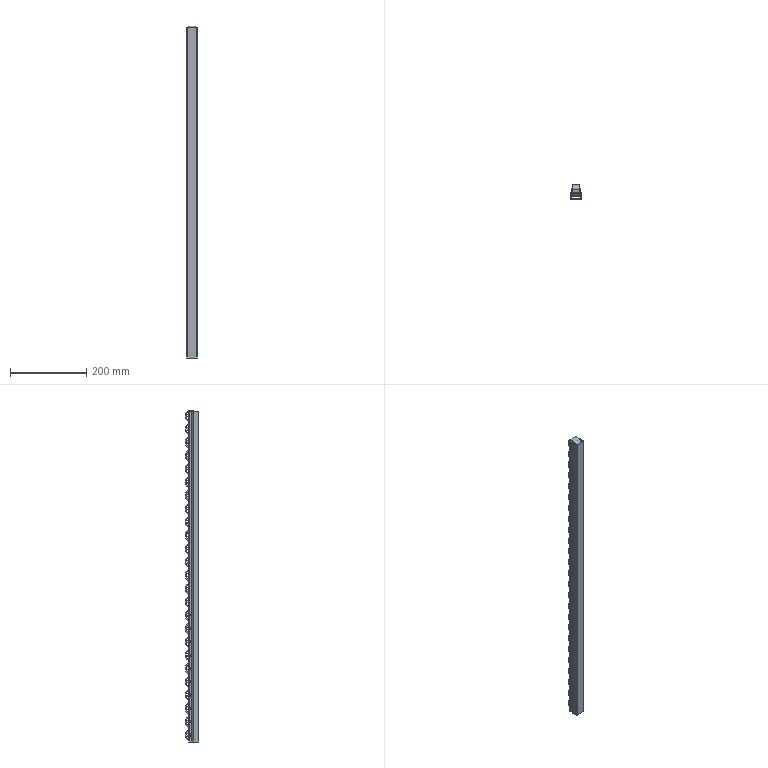Part | STEP file | RIEL FINAL NLV 1 | 35 solids | 1136 faces | box 28.4 x 36.2 x 873.5 mm | volume 257286 mm3 | cylinder 574 | plane 490 | spline 72 | commonest cylinder face diameters 10 x200 25 x200 4 x58 5 x50 30 x50 1.473 x8